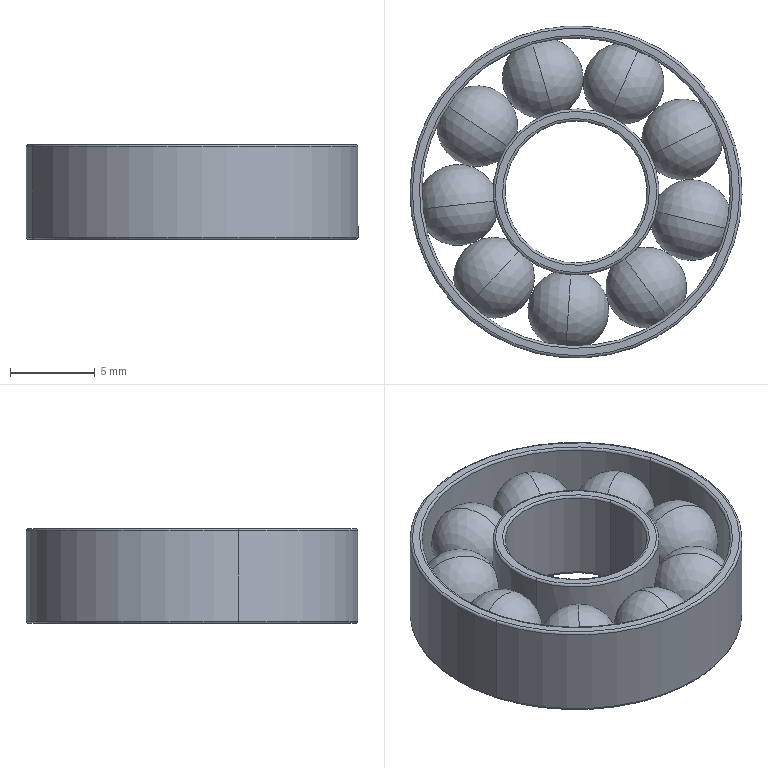Part | SolidWorks | features SplitBody 1 | 1 solid | 46 faces | box 19.6 x 19.6 x 5.6 mm | volume 846.02 mm3 | sphere 18 | torus 16 | cylinder 8 | plane 4 | commonest cylinder face diameters 8.4 x2 9.8 x2 18.2 x2 19.6 x2